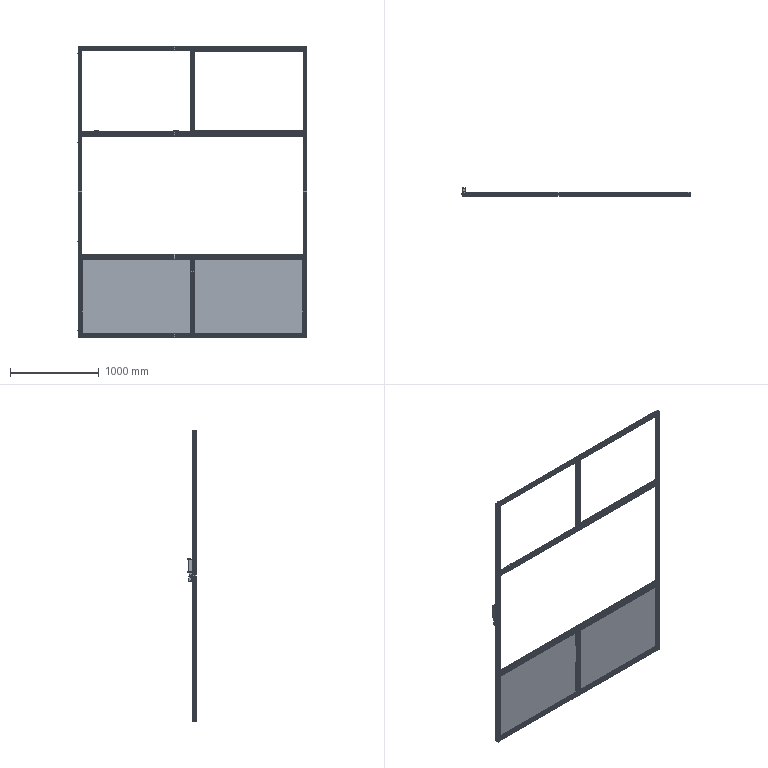Part | SolidWorks | features ReferencePattern 37, LocalLPattern 9, CompositeCurve 6 | 77 solids | 3924 faces | volume 24079558 mm3 | plane 2521 | cylinder 1101 | cone 282 | spline 12 | torus 8 | commonest cylinder face diameters 6.8 x188 2 x108 5 x72 19 x72 1 x56 8 x56